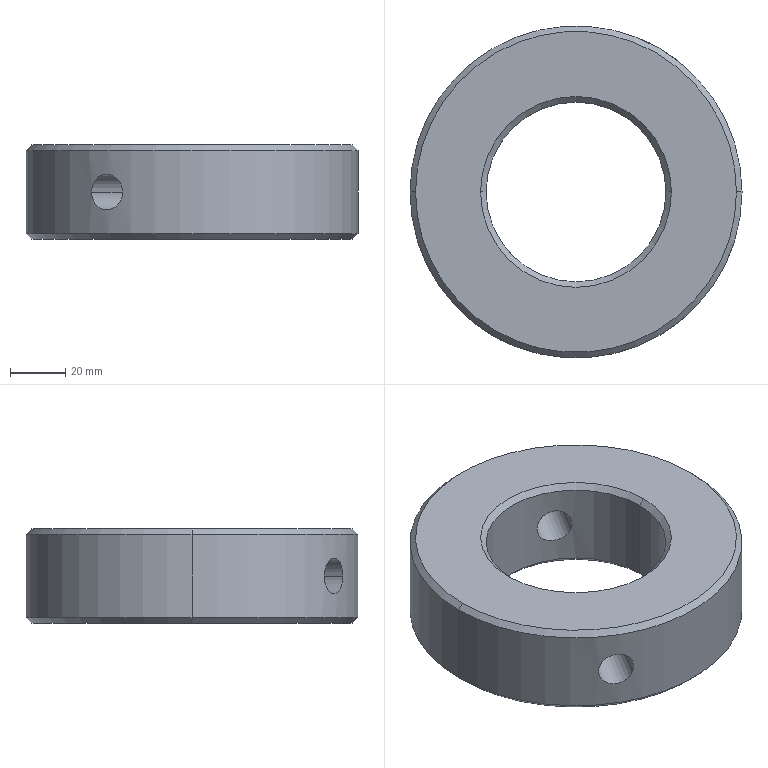Part | SolidWorks | features 3DProfileFeature 1, Chamfer 1, Extrusion 1, HoleWzd 1 | 1 solid | 18 faces | box 120 x 120 x 34 mm | volume 262064 mm3 | cone 8 | cylinder 8 | plane 2 | commonest cylinder face diameters 13 x4 65 x2 120 x2
STEP:
#1=CARTESIAN_POINT('',(-32.5,0.,32.));
#2=VERTEX_POINT('',#1);
#3=CARTESIAN_POINT('',(32.5,0.,32.));
#4=VERTEX_POINT('',#3);
#5=CARTESIAN_POINT('',(0.,0.,32.));
#6=DIRECTION('',(0.,0.,1.));
#7=DIRECTION('',(1.,0.,0.));
#8=AXIS2_PLACEMENT_3D('',#5,#6,#7);
#9=CIRCLE('',#8,32.5);
#10=EDGE_CURVE('',#2,#4,#9,.T.);
#11=ORIENTED_EDGE('',*,*,#10,.F.);
#12=CARTESIAN_POINT('',(-34.5,0.,34.));
#13=VERTEX_POINT('',#12);
#14=CARTESIAN_POINT('',(-32.5,0.,32.));
#15=DIRECTION('',(-0.7071,0.,0.7071));
#16=VECTOR('',#15,1000.);
#17=LINE('',#14,#16);
#18=EDGE_CURVE('',#2,#13,#17,.T.);
#19=ORIENTED_EDGE('',*,*,#18,.T.);
#20=CARTESIAN_POINT('',(34.5,0.,34.));
#21=VERTEX_POINT('',#20);
#22=CARTESIAN_POINT('',(0.,0.,34.));
#23=DIRECTION('',(0.,0.,-1.));
#24=DIRECTION('',(1.,0.,0.));
#25=AXIS2_PLACEMENT_3D('',#22,#23,#24);
#26=CIRCLE('',#25,34.5);
#27=EDGE_CURVE('',#21,#13,#26,.T.);
#28=ORIENTED_EDGE('',*,*,#27,.F.);
#29=CARTESIAN_POINT('',(32.5,0.,32.));
#30=DIRECTION('',(0.7071,0.,0.7071));
#31=VECTOR('',#30,1000.);
#32=LINE('',#29,#31);
#33=EDGE_CURVE('',#4,#21,#32,.T.);
#34=ORIENTED_EDGE('',*,*,#33,.F.);
#35=EDGE_LOOP('',(#11,#19,#28,#34));
#36=FACE_OUTER_BOUND('',#35,.T.);
#37=CARTESIAN_POINT('',(0.,0.,32.));
#38=DIRECTION('',(0.,0.,1.));
#39=DIRECTION('',(1.,0.,0.));
#40=AXIS2_PLACEMENT_3D('',#37,#38,#39);
#41=CONICAL_SURFACE('',#40,32.5,0.7854);
#42=ADVANCED_FACE('',(#36),#41,.F.);
#43=CARTESIAN_POINT('',(32.5,0.,2.));
#44=VERTEX_POINT('',#43);
#45=CARTESIAN_POINT('',(-32.5,0.,2.));
#46=VERTEX_POINT('',#45);
#47=CARTESIAN_POINT('',(0.,0.,2.));
#48=DIRECTION('',(0.,0.,-1.));
#49=DIRECTION('',(1.,0.,0.));
#50=AXIS2_PLACEMENT_3D('',#47,#48,#49);
#51=CIRCLE('',#50,32.5);
#52=EDGE_CURVE('',#44,#46,#51,.T.);
#53=ORIENTED_EDGE('',*,*,#52,.F.);
#54=CARTESIAN_POINT('',(34.5,0.,0.));
#55=VERTEX_POINT('',#54);
#56=CARTESIAN_POINT('',(34.5,0.,0.));
#57=DIRECTION('',(0.7071,0.,-0.7071));
#58=VECTOR('',#57,1000.);
#59=LINE('',#56,#58);
#60=EDGE_CURVE('',#44,#55,#59,.T.);
#61=ORIENTED_EDGE('',*,*,#60,.T.);
#62=CARTESIAN_POINT('',(-34.5,0.,0.));
#63=VERTEX_POINT('',#62);
#64=CARTESIAN_POINT('',(0.,0.,0.));
#65=DIRECTION('',(0.,0.,1.));
#66=DIRECTION('',(1.,0.,0.));
#67=AXIS2_PLACEMENT_3D('',#64,#65,#66);
#68=CIRCLE('',#67,34.5);
#69=EDGE_CURVE('',#63,#55,#68,.T.);
#70=ORIENTED_EDGE('',*,*,#69,.F.);
#71=CARTESIAN_POINT('',(-34.5,0.,0.));
#72=DIRECTION('',(-0.7071,0.,-0.7071));
#73=VECTOR('',#72,1000.);
#74=LINE('',#71,#73);
#75=EDGE_CURVE('',#46,#63,#74,.T.);
#76=ORIENTED_EDGE('',*,*,#75,.F.);
#77=EDGE_LOOP('',(#53,#61,#70,#76));
#78=FACE_OUTER_BOUND('',#77,.T.);
#79=CARTESIAN_POINT('',(0.,0.,0.));
#80=DIRECTION('',(0.,0.,-1.));
#81=DIRECTION('',(-1.,0.,0.));
#82=AXIS2_PLACEMENT_3D('',#79,#80,#81);
#83=CONICAL_SURFACE('',#82,34.5,0.7854);
#84=ADVANCED_FACE('',(#78),#83,.F.);
#85=CARTESIAN_POINT('',(58.,0.,34.));
#86=VERTEX_POINT('',#85);
#87=CARTESIAN_POINT('',(-58.,0.,34.));
#88=VERTEX_POINT('',#87);
#89=CARTESIAN_POINT('',(0.,0.,34.));
#90=DIRECTION('',(0.,0.,1.));
#91=DIRECTION('',(1.,0.,0.));
#92=AXIS2_PLACEMENT_3D('',#89,#90,#91);
#93=CIRCLE('',#92,58.);
#94=EDGE_CURVE('',#86,#88,#93,.T.);
#95=ORIENTED_EDGE('',*,*,#94,.F.);
#96=CARTESIAN_POINT('',(60.,0.,32.));
#97=VERTEX_POINT('',#96);
#98=CARTESIAN_POINT('',(58.,0.,34.));
#99=DIRECTION('',(0.7071,0.,-0.7071));
#100=VECTOR('',#99,1000.);
#101=LINE('',#98,#100);
#102=EDGE_CURVE('',#86,#97,#101,.T.);
#103=ORIENTED_EDGE('',*,*,#102,.T.);
#104=CARTESIAN_POINT('',(-60.,0.,32.));
#105=VERTEX_POINT('',#104);
#106=CARTESIAN_POINT('',(0.,0.,32.));
#107=DIRECTION('',(0.,0.,-1.));
#108=DIRECTION('',(1.,0.,0.));
#109=AXIS2_PLACEMENT_3D('',#106,#107,#108);
#110=CIRCLE('',#109,60.);
#111=EDGE_CURVE('',#105,#97,#110,.T.);
#112=ORIENTED_EDGE('',*,*,#111,.F.);
#113=CARTESIAN_POINT('',(-58.,0.,34.));
#114=DIRECTION('',(-0.7071,0.,-0.7071));
#115=VECTOR('',#114,1000.);
#116=LINE('',#113,#115);
#117=EDGE_CURVE('',#88,#105,#116,.T.);
#118=ORIENTED_EDGE('',*,*,#117,.F.);
#119=EDGE_LOOP('',(#95,#103,#112,#118));
#120=FACE_OUTER_BOUND('',#119,.T.);
#121=CARTESIAN_POINT('',(0.,0.,34.));
#122=DIRECTION('',(0.,0.,-1.));
#123=DIRECTION('',(-1.,0.,0.));
#124=AXIS2_PLACEMENT_3D('',#121,#122,#123);
#125=CONICAL_SURFACE('',#124,58.,0.7854);
#126=ADVANCED_FACE('',(#120),#125,.T.);
#127=CARTESIAN_POINT('',(-58.,0.,0.));
#128=VERTEX_POINT('',#127);
#129=CARTESIAN_POINT('',(58.,0.,0.));
#130=VERTEX_POINT('',#129);
#131=CARTESIAN_POINT('',(0.,0.,0.));
#132=DIRECTION('',(0.,0.,-1.));
#133=DIRECTION('',(1.,0.,0.));
#134=AXIS2_PLACEMENT_3D('',#131,#132,#133);
#135=CIRCLE('',#134,58.);
#136=EDGE_CURVE('',#128,#130,#135,.T.);
#137=ORIENTED_EDGE('',*,*,#136,.F.);
#138=CARTESIAN_POINT('',(-60.,0.,2.));
#139=VERTEX_POINT('',#138);
#140=CARTESIAN_POINT('',(-60.,0.,2.));
#141=DIRECTION('',(-0.7071,0.,0.7071));
#142=VECTOR('',#141,1000.);
#143=LINE('',#140,#142);
#144=EDGE_CURVE('',#128,#139,#143,.T.);
#145=ORIENTED_EDGE('',*,*,#144,.T.);
#146=CARTESIAN_POINT('',(60.,0.,2.));
#147=VERTEX_POINT('',#146);
#148=CARTESIAN_POINT('',(0.,0.,2.));
#149=DIRECTION('',(0.,0.,1.));
#150=DIRECTION('',(1.,0.,0.));
#151=AXIS2_PLACEMENT_3D('',#148,#149,#150);
#152=CIRCLE('',#151,60.);
#153=EDGE_CURVE('',#147,#139,#152,.T.);
#154=ORIENTED_EDGE('',*,*,#153,.F.);
#155=CARTESIAN_POINT('',(60.,0.,2.));
#156=DIRECTION('',(0.7071,0.,0.7071));
#157=VECTOR('',#156,1000.);
#158=LINE('',#155,#157);
#159=EDGE_CURVE('',#130,#147,#158,.T.);
#160=ORIENTED_EDGE('',*,*,#159,.F.);
#161=EDGE_LOOP('',(#137,#145,#154,#160));
#162=FACE_OUTER_BOUND('',#161,.T.);
#163=CARTESIAN_POINT('',(0.,0.,2.));
#164=DIRECTION('',(0.,0.,1.));
#165=DIRECTION('',(1.,0.,0.));
#166=AXIS2_PLACEMENT_3D('',#163,#164,#165);
#167=CONICAL_SURFACE('',#166,60.,0.7854);
#168=ADVANCED_FACE('',(#162),#167,.T.);
#169=CARTESIAN_POINT('',(-25.097,-54.499,17.));
#170=VERTEX_POINT('',#169);
#171=CARTESIAN_POINT('',(-36.247,-47.814,17.));
#172=VERTEX_POINT('',#171);
#173=CARTESIAN_POINT('',(-25.097,-54.499,17.));
#174=CARTESIAN_POINT('',(-25.097,-54.499,16.576));
#175=CARTESIAN_POINT('',(-25.135,-54.482,16.154));
#176=CARTESIAN_POINT('',(-25.249,-54.429,15.525));
#177=CARTESIAN_POINT('',(-25.297,-54.407,15.316));
#178=CARTESIAN_POINT('',(-25.409,-54.354,14.909));
#179=CARTESIAN_POINT('',(-25.54,-54.293,14.51));
#180=CARTESIAN_POINT('',(-25.704,-54.215,14.126));
#181=CARTESIAN_POINT('',(-25.886,-54.129,13.751));
#182=CARTESIAN_POINT('',(-25.986,-54.081,13.567));
#183=CARTESIAN_POINT('',(-26.308,-53.926,13.034));
#184=CARTESIAN_POINT('',(-26.55,-53.807,12.707));
#185=CARTESIAN_POINT('',(-27.087,-53.539,12.107));
#186=CARTESIAN_POINT('',(-27.385,-53.387,11.833));
#187=CARTESIAN_POINT('',(-28.013,-53.06,11.361));
#188=CARTESIAN_POINT('',(-28.343,-52.885,11.161));
#189=CARTESIAN_POINT('',(-28.861,-52.603,10.916));
#190=CARTESIAN_POINT('',(-29.039,-52.505,10.843));
#191=CARTESIAN_POINT('',(-29.396,-52.306,10.719));
#192=CARTESIAN_POINT('',(-29.575,-52.205,10.667));
#193=CARTESIAN_POINT('',(-30.117,-51.896,10.543));
#194=CARTESIAN_POINT('',(-30.481,-51.683,10.5));
#195=CARTESIAN_POINT('',(-31.218,-51.241,10.5));
#196=CARTESIAN_POINT('',(-31.578,-51.019,10.542));
#197=CARTESIAN_POINT('',(-32.106,-50.688,10.665));
#198=CARTESIAN_POINT('',(-32.28,-50.577,10.716));
#199=CARTESIAN_POINT('',(-32.624,-50.356,10.84));
#200=CARTESIAN_POINT('',(-32.794,-50.245,10.912));
#201=CARTESIAN_POINT('',(-33.288,-49.921,11.157));
#202=CARTESIAN_POINT('',(-33.598,-49.712,11.356));
#203=CARTESIAN_POINT('',(-34.182,-49.312,11.827));
#204=CARTESIAN_POINT('',(-34.457,-49.12,12.101));
#205=CARTESIAN_POINT('',(-34.948,-48.772,12.7));
#206=CARTESIAN_POINT('',(-35.167,-48.614,13.027));
#207=CARTESIAN_POINT('',(-35.456,-48.403,13.559));
#208=CARTESIAN_POINT('',(-35.546,-48.337,13.743));
#209=CARTESIAN_POINT('',(-35.708,-48.218,14.118));
#210=CARTESIAN_POINT('',(-35.781,-48.163,14.31));
#211=CARTESIAN_POINT('',(-35.978,-48.017,14.896));
#212=CARTESIAN_POINT('',(-36.078,-47.941,15.305));
#213=CARTESIAN_POINT('',(-36.213,-47.839,16.145));
#214=CARTESIAN_POINT('',(-36.247,-47.814,16.57));
#215=CARTESIAN_POINT('',(-36.247,-47.814,17.));
#216=B_SPLINE_CURVE_WITH_KNOTS('',3,(#173,#174,#175,#176,#177,#178,#179,#180,#181,#182,#183,#184,#185,#186,#187,#188,#189,#190,#191,#192,#193,#194,#195,#196,#197,#198,#199,#200,#201,#202,#203,#204,#205,#206,#207,#208,#209,#210,#211,#212,#213,#214,#215),.UNSPECIFIED.,.F.,.F.,(4,2,2,1,2,2,2,2,2,2,2,2,2,2,2,2,2,2,2,2,2,4),(0.02034,0.02161,0.02224,0.02288,0.02351,0.02415,0.02542,0.02669,0.02796,0.0286,0.02923,0.0305,0.03177,0.03241,0.03304,0.03432,0.03559,0.03686,0.03749,0.03813,0.0394,0.04067),.UNSPECIFIED.);
#217=EDGE_CURVE('',#170,#172,#216,.T.);
#218=ORIENTED_EDGE('',*,*,#217,.F.);
#219=CARTESIAN_POINT('',(-10.8,-30.653,17.));
#220=VERTEX_POINT('',#219);
#221=CARTESIAN_POINT('',(36.429,48.117,17.));
#222=DIRECTION('',(0.5142,0.8577,0.));
#223=VECTOR('',#222,1000.);
#224=LINE('',#221,#223);
#225=EDGE_CURVE('',#170,#220,#224,.T.);
#226=ORIENTED_EDGE('',*,*,#225,.T.);
#227=CARTESIAN_POINT('',(-21.95,-23.968,17.));
#228=VERTEX_POINT('',#227);
#229=CARTESIAN_POINT('',(-10.8,-30.653,17.));
#230=CARTESIAN_POINT('',(-10.8,-30.653,16.575));
#231=CARTESIAN_POINT('',(-10.84,-30.639,16.152));
#232=CARTESIAN_POINT('',(-11.001,-30.582,15.31));
#233=CARTESIAN_POINT('',(-11.12,-30.539,14.902));
#234=CARTESIAN_POINT('',(-11.352,-30.453,14.315));
#235=CARTESIAN_POINT('',(-11.439,-30.421,14.124));
#236=CARTESIAN_POINT('',(-11.629,-30.348,13.748));
#237=CARTESIAN_POINT('',(-11.734,-30.308,13.563));
#238=CARTESIAN_POINT('',(-12.069,-30.177,13.033));
#239=CARTESIAN_POINT('',(-12.321,-30.075,12.706));
#240=CARTESIAN_POINT('',(-12.879,-29.841,12.107));
#241=CARTESIAN_POINT('',(-13.187,-29.707,11.833));
#242=CARTESIAN_POINT('',(-13.831,-29.412,11.362));
#243=CARTESIAN_POINT('',(-14.169,-29.251,11.162));
#244=CARTESIAN_POINT('',(-14.7,-28.986,10.916));
#245=CARTESIAN_POINT('',(-14.881,-28.894,10.843));
#246=CARTESIAN_POINT('',(-15.243,-28.705,10.719));
#247=CARTESIAN_POINT('',(-15.424,-28.607,10.668));
#248=CARTESIAN_POINT('',(-15.972,-28.308,10.543));
#249=CARTESIAN_POINT('',(-16.342,-28.096,10.5));
#250=CARTESIAN_POINT('',(-17.078,-27.655,10.5));
#251=CARTESIAN_POINT('',(-17.436,-27.43,10.542));
#252=CARTESIAN_POINT('',(-18.134,-26.974,10.707));
#253=CARTESIAN_POINT('',(-18.477,-26.74,10.833));
#254=CARTESIAN_POINT('',(-19.119,-26.284,11.158));
#255=CARTESIAN_POINT('',(-19.421,-26.062,11.357));
#256=CARTESIAN_POINT('',(-19.845,-25.738,11.712));
#257=CARTESIAN_POINT('',(-19.983,-25.631,11.84));
#258=CARTESIAN_POINT('',(-20.243,-25.426,12.11));
#259=CARTESIAN_POINT('',(-20.367,-25.327,12.252));
#260=CARTESIAN_POINT('',(-20.719,-25.042,12.7));
#261=CARTESIAN_POINT('',(-20.928,-24.866,13.026));
#262=CARTESIAN_POINT('',(-21.295,-24.552,13.738));
#263=CARTESIAN_POINT('',(-21.448,-24.418,14.112));
#264=CARTESIAN_POINT('',(-21.634,-24.254,14.698));
#265=CARTESIAN_POINT('',(-21.688,-24.205,14.898));
#266=CARTESIAN_POINT('',(-21.783,-24.12,15.306));
#267=CARTESIAN_POINT('',(-21.823,-24.084,15.515));
#268=CARTESIAN_POINT('',(-21.918,-23.997,16.145));
#269=CARTESIAN_POINT('',(-21.95,-23.968,16.569));
#270=CARTESIAN_POINT('',(-21.95,-23.968,17.));
#271=B_SPLINE_CURVE_WITH_KNOTS('',3,(#229,#230,#231,#232,#233,#234,#235,#236,#237,#238,#239,#240,#241,#242,#243,#244,#245,#246,#247,#248,#249,#250,#251,#252,#253,#254,#255,#256,#257,#258,#259,#260,#261,#262,#263,#264,#265,#266,#267,#268,#269,#270),.UNSPECIFIED.,.F.,.F.,(4,2,2,2,2,2,2,2,2,2,2,2,2,2,2,2,2,2,2,2,4),(0.02037,0.02165,0.02292,0.02356,0.02419,0.02547,0.02674,0.02801,0.02865,0.02928,0.03056,0.03183,0.0331,0.03438,0.03501,0.03565,0.03692,0.0382,0.03883,0.03947,0.04074),.UNSPECIFIED.);
#272=EDGE_CURVE('',#220,#228,#271,.T.);
#273=ORIENTED_EDGE('',*,*,#272,.T.);
#274=CARTESIAN_POINT('',(25.279,54.802,17.));
#275=DIRECTION('',(0.5142,0.8577,0.));
#276=VECTOR('',#275,1000.);
#277=LINE('',#274,#276);
#278=EDGE_CURVE('',#172,#228,#277,.T.);
#279=ORIENTED_EDGE('',*,*,#278,.F.);
#280=EDGE_LOOP('',(#218,#226,#273,#279));
#281=FACE_OUTER_BOUND('',#280,.T.);
#282=CARTESIAN_POINT('',(30.854,51.459,17.));
#283=DIRECTION('',(0.5142,0.8577,0.));
#284=DIRECTION('',(-0.8577,0.5142,0.));
#285=AXIS2_PLACEMENT_3D('',#282,#283,#284);
#286=CYLINDRICAL_SURFACE('',#285,6.5);
#287=ADVANCED_FACE('',(#281),#286,.F.);
#288=CARTESIAN_POINT('',(10.8,30.653,17.));
#289=VERTEX_POINT('',#288);
#290=CARTESIAN_POINT('',(21.95,23.968,17.));
#291=VERTEX_POINT('',#290);
#292=CARTESIAN_POINT('',(10.8,30.653,17.));
#293=CARTESIAN_POINT('',(10.8,30.653,16.569));
#294=CARTESIAN_POINT('',(10.841,30.639,16.146));
#295=CARTESIAN_POINT('',(10.96,30.596,15.522));
#296=CARTESIAN_POINT('',(11.01,30.578,15.316));
#297=CARTESIAN_POINT('',(11.129,30.535,14.907));
#298=CARTESIAN_POINT('',(11.199,30.51,14.704));
#299=CARTESIAN_POINT('',(11.432,30.423,14.114));
#300=CARTESIAN_POINT('',(11.622,30.352,13.741));
#301=CARTESIAN_POINT('',(12.068,30.177,13.035));
#302=CARTESIAN_POINT('',(12.325,30.074,12.702));
#303=CARTESIAN_POINT('',(12.882,29.84,12.104));
#304=CARTESIAN_POINT('',(13.184,29.708,11.835));
#305=CARTESIAN_POINT('',(13.834,29.411,11.36));
#306=CARTESIAN_POINT('',(14.176,29.248,11.159));
#307=CARTESIAN_POINT('',(14.702,28.985,10.915));
#308=CARTESIAN_POINT('',(14.88,28.894,10.844));
#309=CARTESIAN_POINT('',(15.242,28.705,10.72));
#310=CARTESIAN_POINT('',(15.426,28.606,10.667));
#311=CARTESIAN_POINT('',(15.979,28.304,10.542));
#312=CARTESIAN_POINT('',(16.346,28.094,10.5));
#313=CARTESIAN_POINT('',(17.075,27.656,10.5));
#314=CARTESIAN_POINT('',(17.441,27.427,10.542));
#315=CARTESIAN_POINT('',(18.14,26.97,10.709));
#316=CARTESIAN_POINT('',(18.476,26.741,10.832));
#317=CARTESIAN_POINT('',(18.959,26.398,11.077));
#318=CARTESIAN_POINT('',(19.118,26.283,11.169));
#319=CARTESIAN_POINT('',(19.421,26.059,11.37));
#320=CARTESIAN_POINT('',(19.567,25.95,11.48));
#321=CARTESIAN_POINT('',(19.989,25.628,11.832));
#322=CARTESIAN_POINT('',(20.25,25.422,12.102));
#323=CARTESIAN_POINT('',(20.724,25.037,12.706));
#324=CARTESIAN_POINT('',(20.932,24.863,13.034));
#325=CARTESIAN_POINT('',(21.204,24.631,13.561));
#326=CARTESIAN_POINT('',(21.288,24.558,13.743));
#327=CARTESIAN_POINT('',(21.442,24.423,14.119));
#328=CARTESIAN_POINT('',(21.512,24.361,14.314));
#329=CARTESIAN_POINT('',(21.698,24.196,14.903));
#330=CARTESIAN_POINT('',(21.791,24.112,15.308));
#331=CARTESIAN_POINT('',(21.886,24.026,15.935));
#332=CARTESIAN_POINT('',(21.91,24.004,16.148));
#333=CARTESIAN_POINT('',(21.942,23.975,16.575));
#334=CARTESIAN_POINT('',(21.95,23.968,16.788));
#335=CARTESIAN_POINT('',(21.95,23.968,17.));
#336=B_SPLINE_CURVE_WITH_KNOTS('',3,(#292,#293,#294,#295,#296,#297,#298,#299,#300,#301,#302,#303,#304,#305,#306,#307,#308,#309,#310,#311,#312,#313,#314,#315,#316,#317,#318,#319,#320,#321,#322,#323,#324,#325,#326,#327,#328,#329,#330,#331,#332,#333,#334,#335),.UNSPECIFIED.,.F.,.F.,(4,2,2,2,2,2,2,2,2,2,2,2,2,2,2,2,2,2,2,2,2,4),(0.,0.001273,0.00191,0.002547,0.00382,0.005093,0.006367,0.00764,0.008277,0.008913,0.01019,0.01146,0.01273,0.01337,0.01401,0.01528,0.01655,0.01719,0.01783,0.0191,0.01974,0.02037),.UNSPECIFIED.);
#337=EDGE_CURVE('',#289,#291,#336,.T.);
#338=ORIENTED_EDGE('',*,*,#337,.T.);
#339=CARTESIAN_POINT('',(36.247,47.814,17.));
#340=VERTEX_POINT('',#339);
#341=CARTESIAN_POINT('',(36.429,48.117,17.));
#342=DIRECTION('',(0.5142,0.8577,0.));
#343=VECTOR('',#342,1000.);
#344=LINE('',#341,#343);
#345=EDGE_CURVE('',#291,#340,#344,.T.);
#346=ORIENTED_EDGE('',*,*,#345,.T.);
#347=CARTESIAN_POINT('',(25.097,54.499,17.));
#348=VERTEX_POINT('',#347);
#349=CARTESIAN_POINT('',(25.097,54.499,17.));
#350=CARTESIAN_POINT('',(25.097,54.499,16.57));
#351=CARTESIAN_POINT('',(25.136,54.481,16.148));
#352=CARTESIAN_POINT('',(25.249,54.429,15.524));
#353=CARTESIAN_POINT('',(25.296,54.407,15.318));
#354=CARTESIAN_POINT('',(25.409,54.354,14.91));
#355=CARTESIAN_POINT('',(25.475,54.323,14.707));
#356=CARTESIAN_POINT('',(25.698,54.218,14.116));
#357=CARTESIAN_POINT('',(25.879,54.132,13.743));
#358=CARTESIAN_POINT('',(26.306,53.926,13.037));
#359=CARTESIAN_POINT('',(26.553,53.805,12.702));
#360=CARTESIAN_POINT('',(27.091,53.537,12.103));
#361=CARTESIAN_POINT('',(27.383,53.388,11.834));
#362=CARTESIAN_POINT('',(27.857,53.142,11.478));
#363=CARTESIAN_POINT('',(28.02,53.056,11.367));
#364=CARTESIAN_POINT('',(28.352,52.879,11.167));
#365=CARTESIAN_POINT('',(28.69,52.698,10.986));
#366=CARTESIAN_POINT('',(29.039,52.505,10.843));
#367=CARTESIAN_POINT('',(29.395,52.307,10.719));
#368=CARTESIAN_POINT('',(29.577,52.204,10.667));
#369=CARTESIAN_POINT('',(30.124,51.892,10.541));
#370=CARTESIAN_POINT('',(30.488,51.679,10.5));
#371=CARTESIAN_POINT('',(31.216,51.242,10.5));
#372=CARTESIAN_POINT('',(31.583,51.017,10.542));
#373=CARTESIAN_POINT('',(32.289,50.573,10.708));
#374=CARTESIAN_POINT('',(32.63,50.353,10.831));
#375=CARTESIAN_POINT('',(33.124,50.028,11.076));
#376=CARTESIAN_POINT('',(33.286,49.92,11.168));
#377=CARTESIAN_POINT('',(33.599,49.71,11.369));
#378=CARTESIAN_POINT('',(33.75,49.608,11.478));
#379=CARTESIAN_POINT('',(34.186,49.309,11.831));
#380=CARTESIAN_POINT('',(34.456,49.121,12.1));
#381=CARTESIAN_POINT('',(34.953,48.769,12.707));
#382=CARTESIAN_POINT('',(35.171,48.611,13.035));
#383=CARTESIAN_POINT('',(35.458,48.402,13.562));
#384=CARTESIAN_POINT('',(35.546,48.337,13.744));
#385=CARTESIAN_POINT('',(35.709,48.217,14.12));
#386=CARTESIAN_POINT('',(35.783,48.162,14.315));
#387=CARTESIAN_POINT('',(35.981,48.015,14.906));
#388=CARTESIAN_POINT('',(36.079,47.94,15.311));
#389=CARTESIAN_POINT('',(36.213,47.84,16.145));
#390=CARTESIAN_POINT('',(36.247,47.814,16.576));
#391=CARTESIAN_POINT('',(36.247,47.814,17.));
#392=B_SPLINE_CURVE_WITH_KNOTS('',3,(#349,#350,#351,#352,#353,#354,#355,#356,#357,#358,#359,#360,#361,#362,#363,#364,#365,#366,#367,#368,#369,#370,#371,#372,#373,#374,#375,#376,#377,#378,#379,#380,#381,#382,#383,#384,#385,#386,#387,#388,#389,#390,#391),.UNSPECIFIED.,.F.,.F.,(4,2,2,2,2,2,2,2,1,2,2,2,2,2,2,2,2,2,2,2,2,4),(0.,0.001271,0.001907,0.002542,0.003813,0.005084,0.006355,0.006991,0.007626,0.008262,0.008897,0.01017,0.01144,0.01271,0.01335,0.01398,0.01525,0.01652,0.01716,0.01779,0.01907,0.02034),.UNSPECIFIED.);
#393=EDGE_CURVE('',#348,#340,#392,.T.);
#394=ORIENTED_EDGE('',*,*,#393,.F.);
#395=CARTESIAN_POINT('',(25.279,54.802,17.));
#396=DIRECTION('',(0.5142,0.8577,0.));
#397=VECTOR('',#396,1000.);
#398=LINE('',#395,#397);
#399=EDGE_CURVE('',#289,#348,#398,.T.);
#400=ORIENTED_EDGE('',*,*,#399,.F.);
#401=EDGE_LOOP('',(#338,#346,#394,#400));
#402=FACE_OUTER_BOUND('',#401,.T.);
#403=CARTESIAN_POINT('',(30.854,51.459,17.));
#404=DIRECTION('',(0.5142,0.8577,0.));
#405=DIRECTION('',(-0.8577,0.5142,0.));
#406=AXIS2_PLACEMENT_3D('',#403,#404,#405);
#407=CYLINDRICAL_SURFACE('',#406,6.5);
#408=ADVANCED_FACE('',(#402),#407,.F.);
#409=CARTESIAN_POINT('',(-21.95,-23.968,17.));
#410=CARTESIAN_POINT('',(-21.95,-23.968,17.431));
#411=CARTESIAN_POINT('',(-21.918,-23.997,17.854));
#412=CARTESIAN_POINT('',(-21.824,-24.083,18.478));
#413=CARTESIAN_POINT('',(-21.785,-24.118,18.684));
#414=CARTESIAN_POINT('',(-21.691,-24.203,19.093));
#415=CARTESIAN_POINT('',(-21.635,-24.252,19.296));
#416=CARTESIAN_POINT('',(-21.449,-24.418,19.886));
#417=CARTESIAN_POINT('',(-21.296,-24.551,20.259));
#418=CARTESIAN_POINT('',(-20.933,-24.862,20.965));
#419=CARTESIAN_POINT('',(-20.72,-25.04,21.298));
#420=CARTESIAN_POINT('',(-20.251,-25.421,21.896));
#421=CARTESIAN_POINT('',(-19.993,-25.625,22.165));
#422=CARTESIAN_POINT('',(-19.425,-26.059,22.64));
#423=CARTESIAN_POINT('',(-19.12,-26.284,22.841));
#424=CARTESIAN_POINT('',(-18.64,-26.624,23.085));
#425=CARTESIAN_POINT('',(-18.476,-26.738,23.156));
#426=CARTESIAN_POINT('',(-18.139,-26.968,23.28));
#427=CARTESIAN_POINT('',(-17.965,-27.084,23.333));
#428=CARTESIAN_POINT('',(-17.437,-27.429,23.458));
#429=CARTESIAN_POINT('',(-17.079,-27.654,23.5));
#430=CARTESIAN_POINT('',(-16.35,-28.091,23.5));
#431=CARTESIAN_POINT('',(-15.975,-28.306,23.458));
#432=CARTESIAN_POINT('',(-15.243,-28.707,23.291));
#433=CARTESIAN_POINT('',(-14.882,-28.895,23.168));
#434=CARTESIAN_POINT('',(-14.352,-29.16,22.923));
#435=CARTESIAN_POINT('',(-14.176,-29.246,22.831));
#436=CARTESIAN_POINT('',(-13.836,-29.408,22.63));
#437=CARTESIAN_POINT('',(-13.67,-29.486,22.52));
#438=CARTESIAN_POINT('',(-13.188,-29.706,22.168));
#439=CARTESIAN_POINT('',(-12.883,-29.839,21.898));
#440=CARTESIAN_POINT('',(-12.321,-30.076,21.294));
#441=CARTESIAN_POINT('',(-12.069,-30.177,20.966));
#442=CARTESIAN_POINT('',(-11.736,-30.307,20.439));
#443=CARTESIAN_POINT('',(-11.632,-30.347,20.257));
#444=CARTESIAN_POINT('',(-11.441,-30.42,19.881));
#445=CARTESIAN_POINT('',(-11.353,-30.453,19.686));
#446=CARTESIAN_POINT('',(-11.12,-30.539,19.097));
#447=CARTESIAN_POINT('',(-11.001,-30.581,18.692));
#448=CARTESIAN_POINT('',(-10.881,-30.624,18.065));
#449=CARTESIAN_POINT('',(-10.851,-30.635,17.852));
#450=CARTESIAN_POINT('',(-10.81,-30.65,17.425));
#451=CARTESIAN_POINT('',(-10.8,-30.653,17.212));
#452=CARTESIAN_POINT('',(-10.8,-30.653,17.));
#453=B_SPLINE_CURVE_WITH_KNOTS('',3,(#409,#410,#411,#412,#413,#414,#415,#416,#417,#418,#419,#420,#421,#422,#423,#424,#425,#426,#427,#428,#429,#430,#431,#432,#433,#434,#435,#436,#437,#438,#439,#440,#441,#442,#443,#444,#445,#446,#447,#448,#449,#450,#451,#452),.UNSPECIFIED.,.F.,.F.,(4,2,2,2,2,2,2,2,2,2,2,2,2,2,2,2,2,2,2,2,2,4),(0.,0.001273,0.00191,0.002547,0.00382,0.005093,0.006367,0.00764,0.008277,0.008913,0.01019,0.01146,0.01273,0.01337,0.01401,0.01528,0.01655,0.01719,0.01783,0.0191,0.01974,0.02037),.UNSPECIFIED.);
#454=EDGE_CURVE('',#228,#220,#453,.T.);
#455=ORIENTED_EDGE('',*,*,#454,.F.);
#456=ORIENTED_EDGE('',*,*,#272,.F.);
#457=EDGE_LOOP('',(#455,#456));
#458=FACE_BOUND('',#457,.T.);
#459=ORIENTED_EDGE('',*,*,#10,.T.);
#460=CARTESIAN_POINT('',(32.5,0.,34.));
#461=DIRECTION('',(0.,0.,-1.));
#462=VECTOR('',#461,1000.);
#463=LINE('',#460,#462);
#464=EDGE_CURVE('',#4,#44,#463,.T.);
#465=ORIENTED_EDGE('',*,*,#464,.T.);
#466=ORIENTED_EDGE('',*,*,#52,.T.);
#467=CARTESIAN_POINT('',(-32.5,0.,34.));
#468=DIRECTION('',(0.,0.,-1.));
#469=VECTOR('',#468,1000.);
#470=LINE('',#467,#469);
#471=EDGE_CURVE('',#2,#46,#470,.T.);
#472=ORIENTED_EDGE('',*,*,#471,.F.);
#473=EDGE_LOOP('',(#459,#465,#466,#472));
#474=FACE_OUTER_BOUND('',#473,.T.);
#475=CARTESIAN_POINT('',(0.,0.,34.));
#476=DIRECTION('',(0.,0.,-1.));
#477=DIRECTION('',(-1.,0.,0.));
#478=AXIS2_PLACEMENT_3D('',#475,#476,#477);
#479=CYLINDRICAL_SURFACE('',#478,32.5);
#480=ADVANCED_FACE('',(#458,#474),#479,.F.);
#481=ORIENTED_EDGE('',*,*,#393,.T.);
#482=CARTESIAN_POINT('',(36.247,47.814,17.));
#483=CARTESIAN_POINT('',(36.247,47.814,17.424));
#484=CARTESIAN_POINT('',(36.214,47.839,17.846));
#485=CARTESIAN_POINT('',(36.114,47.915,18.475));
#486=CARTESIAN_POINT('',(36.072,47.946,18.684));
#487=CARTESIAN_POINT('',(35.972,48.021,19.091));
#488=CARTESIAN_POINT('',(35.857,48.107,19.49));
#489=CARTESIAN_POINT('',(35.711,48.215,19.874));
#490=CARTESIAN_POINT('',(35.549,48.335,20.249));
#491=CARTESIAN_POINT('',(35.46,48.4,20.433));
#492=CARTESIAN_POINT('',(35.171,48.611,20.966));
#493=CARTESIAN_POINT('',(34.953,48.769,21.293));
#494=CARTESIAN_POINT('',(34.463,49.116,21.893));
#495=CARTESIAN_POINT('',(34.188,49.308,22.167));
#496=CARTESIAN_POINT('',(33.605,49.708,22.639));
#497=CARTESIAN_POINT('',(33.295,49.916,22.839));
#498=CARTESIAN_POINT('',(32.802,50.24,23.084));
#499=CARTESIAN_POINT('',(32.631,50.351,23.157));
#500=CARTESIAN_POINT('',(32.288,50.572,23.281));
#501=CARTESIAN_POINT('',(32.114,50.683,23.333));
#502=CARTESIAN_POINT('',(31.586,51.015,23.457));
#503=CARTESIAN_POINT('',(31.226,51.236,23.5));
#504=CARTESIAN_POINT('',(30.49,51.678,23.5));
#505=CARTESIAN_POINT('',(30.125,51.891,23.458));
#506=CARTESIAN_POINT('',(29.583,52.2,23.335));
#507=CARTESIAN_POINT('',(29.404,52.302,23.284));
#508=CARTESIAN_POINT('',(29.047,52.501,23.16));
#509=CARTESIAN_POINT('',(28.869,52.599,23.088));
#510=CARTESIAN_POINT('',(28.35,52.881,22.843));
#511=CARTESIAN_POINT('',(28.02,53.057,22.644));
#512=CARTESIAN_POINT('',(27.392,53.384,22.173));
#513=CARTESIAN_POINT('',(27.093,53.536,21.899));
#514=CARTESIAN_POINT('',(26.555,53.804,21.3));
#515=CARTESIAN_POINT('',(26.312,53.923,20.973));
#516=CARTESIAN_POINT('',(25.99,54.079,20.441));
#517=CARTESIAN_POINT('',(25.89,54.127,20.257));
#518=CARTESIAN_POINT('',(25.708,54.214,19.882));
#519=CARTESIAN_POINT('',(25.625,54.253,19.69));
#520=CARTESIAN_POINT('',(25.404,54.357,19.104));
#521=CARTESIAN_POINT('',(25.289,54.41,18.695));
#522=CARTESIAN_POINT('',(25.136,54.481,17.855));
#523=CARTESIAN_POINT('',(25.097,54.499,17.43));
#524=CARTESIAN_POINT('',(25.097,54.499,17.));
#525=B_SPLINE_CURVE_WITH_KNOTS('',3,(#482,#483,#484,#485,#486,#487,#488,#489,#490,#491,#492,#493,#494,#495,#496,#497,#498,#499,#500,#501,#502,#503,#504,#505,#506,#507,#508,#509,#510,#511,#512,#513,#514,#515,#516,#517,#518,#519,#520,#521,#522,#523,#524),.UNSPECIFIED.,.F.,.F.,(4,2,2,1,2,2,2,2,2,2,2,2,2,2,2,2,2,2,2,2,2,4),(0.02034,0.02161,0.02224,0.02288,0.02351,0.02415,0.02542,0.02669,0.02796,0.0286,0.02923,0.0305,0.03177,0.03241,0.03304,0.03432,0.03559,0.03686,0.03749,0.03813,0.0394,0.04067),.UNSPECIFIED.);
#526=EDGE_CURVE('',#340,#348,#525,.T.);
#527=ORIENTED_EDGE('',*,*,#526,.T.);
#528=EDGE_LOOP('',(#481,#527));
#529=FACE_BOUND('',#528,.T.);
#530=ORIENTED_EDGE('',*,*,#111,.T.);
#531=CARTESIAN_POINT('',(60.,0.,34.));
#532=DIRECTION('',(0.,0.,-1.));
#533=VECTOR('',#532,1000.);
#534=LINE('',#531,#533);
#535=EDGE_CURVE('',#97,#147,#534,.T.);
#536=ORIENTED_EDGE('',*,*,#535,.T.);
#537=ORIENTED_EDGE('',*,*,#153,.T.);
#538=CARTESIAN_POINT('',(-60.,0.,34.));
#539=DIRECTION('',(0.,0.,-1.));
#540=VECTOR('',#539,1000.);
#541=LINE('',#538,#540);
#542=EDGE_CURVE('',#105,#139,#541,.T.);
#543=ORIENTED_EDGE('',*,*,#542,.F.);
#544=EDGE_LOOP('',(#530,#536,#537,#543));
#545=FACE_OUTER_BOUND('',#544,.T.);
#546=CARTESIAN_POINT('',(0.,0.,34.));
#547=DIRECTION('',(0.,0.,-1.));
#548=DIRECTION('',(-1.,0.,0.));
#549=AXIS2_PLACEMENT_3D('',#546,#547,#548);
#550=CYLINDRICAL_SURFACE('',#549,60.);
#551=ADVANCED_FACE('',(#529,#545),#550,.T.);
#552=CARTESIAN_POINT('',(0.,0.,34.));
#553=DIRECTION('',(0.,0.,1.));
#554=DIRECTION('',(1.,0.,0.));
#555=AXIS2_PLACEMENT_3D('',#552,#553,#554);
#556=CIRCLE('',#555,58.);
#557=EDGE_CURVE('',#88,#86,#556,.T.);
#558=ORIENTED_EDGE('',*,*,#557,.T.);
#559=ORIENTED_EDGE('',*,*,#94,.T.);
#560=EDGE_LOOP('',(#558,#559));
#561=FACE_OUTER_BOUND('',#560,.T.);
#562=ORIENTED_EDGE('',*,*,#27,.T.);
#563=CARTESIAN_POINT('',(0.,0.,34.));
#564=DIRECTION('',(0.,0.,-1.));
#565=DIRECTION('',(1.,0.,0.));
#566=AXIS2_PLACEMENT_3D('',#563,#564,#565);
#567=CIRCLE('',#566,34.5);
#568=EDGE_CURVE('',#13,#21,#567,.T.);
#569=ORIENTED_EDGE('',*,*,#568,.T.);
#570=EDGE_LOOP('',(#562,#569));
#571=FACE_BOUND('',#570,.T.);
#572=CARTESIAN_POINT('',(0.,0.,34.));
#573=DIRECTION('',(0.,0.,1.));
#574=DIRECTION('',(1.,0.,0.));
#575=AXIS2_PLACEMENT_3D('',#572,#573,#574);
#576=PLANE('',#575);
#577=ADVANCED_FACE('',(#561,#571),#576,.T.);
#578=CARTESIAN_POINT('',(0.,0.,0.));
#579=DIRECTION('',(0.,0.,-1.));
#580=DIRECTION('',(1.,0.,0.));
#581=AXIS2_PLACEMENT_3D('',#578,#579,#580);
#582=CIRCLE('',#581,58.);
#583=EDGE_CURVE('',#130,#128,#582,.T.);
#584=ORIENTED_EDGE('',*,*,#583,.T.);
#585=ORIENTED_EDGE('',*,*,#136,.T.);
#586=EDGE_LOOP('',(#584,#585));
#587=FACE_OUTER_BOUND('',#586,.T.);
#588=ORIENTED_EDGE('',*,*,#69,.T.);
#589=CARTESIAN_POINT('',(0.,0.,0.));
#590=DIRECTION('',(0.,0.,1.));
#591=DIRECTION('',(1.,0.,0.));
#592=AXIS2_PLACEMENT_3D('',#589,#590,#591);
#593=CIRCLE('',#592,34.5);
#594=EDGE_CURVE('',#55,#63,#593,.T.);
#595=ORIENTED_EDGE('',*,*,#594,.T.);
#596=EDGE_LOOP('',(#588,#595));
#597=FACE_BOUND('',#596,.T.);
#598=CARTESIAN_POINT('',(0.,0.,0.));
#599=DIRECTION('',(0.,0.,1.));
#600=DIRECTION('',(1.,0.,0.));
#601=AXIS2_PLACEMENT_3D('',#598,#599,#600);
#602=PLANE('',#601);
#603=ADVANCED_FACE('',(#587,#597),#602,.F.);
#604=ORIENTED_EDGE('',*,*,#535,.F.);
#605=CARTESIAN_POINT('',(0.,0.,32.));
#606=DIRECTION('',(0.,0.,-1.));
#607=DIRECTION('',(1.,0.,0.));
#608=AXIS2_PLACEMENT_3D('',#605,#606,#607);
#609=CIRCLE('',#608,60.);
#610=EDGE_CURVE('',#97,#105,#609,.T.);
#611=ORIENTED_EDGE('',*,*,#610,.T.);
#612=ORIENTED_EDGE('',*,*,#542,.T.);
#613=CARTESIAN_POINT('',(0.,0.,2.));
#614=DIRECTION('',(0.,0.,1.));
#615=DIRECTION('',(1.,0.,0.));
#616=AXIS2_PLACEMENT_3D('',#613,#614,#615);
#617=CIRCLE('',#616,60.);
#618=EDGE_CURVE('',#139,#147,#617,.T.);
#619=ORIENTED_EDGE('',*,*,#618,.T.);
#620=EDGE_LOOP('',(#604,#611,#612,#619));
#621=FACE_OUTER_BOUND('',#620,.T.);
#622=CARTESIAN_POINT('',(-36.247,-47.814,17.));
#623=CARTESIAN_POINT('',(-36.247,-47.814,17.43));
#624=CARTESIAN_POINT('',(-36.213,-47.839,17.852));
#625=CARTESIAN_POINT('',(-36.114,-47.915,18.476));
#626=CARTESIAN_POINT('',(-36.072,-47.946,18.682));
#627=CARTESIAN_POINT('',(-35.973,-48.021,19.09));
#628=CARTESIAN_POINT('',(-35.914,-48.064,19.293));
#629=CARTESIAN_POINT('',(-35.717,-48.211,19.884));
#630=CARTESIAN_POINT('',(-35.556,-48.331,20.257));
#631=CARTESIAN_POINT('',(-35.173,-48.61,20.963));
#632=CARTESIAN_POINT('',(-34.95,-48.771,21.298));
#633=CARTESIAN_POINT('',(-34.459,-49.119,21.897));
#634=CARTESIAN_POINT('',(-34.19,-49.307,22.166));
#635=CARTESIAN_POINT('',(-33.75,-49.608,22.522));
#636=CARTESIAN_POINT('',(-33.597,-49.712,22.633));
#637=CARTESIAN_POINT('',(-33.285,-49.921,22.833));
#638=CARTESIAN_POINT('',(-32.966,-50.134,23.014));
#639=CARTESIAN_POINT('',(-32.631,-50.351,23.157));
#640=CARTESIAN_POINT('',(-32.289,-50.572,23.281));
#641=CARTESIAN_POINT('',(-32.112,-50.684,23.333));
#642=CARTESIAN_POINT('',(-31.579,-51.019,23.459));
#643=CARTESIAN_POINT('',(-31.22,-51.24,23.5));
#644=CARTESIAN_POINT('',(-30.492,-51.676,23.5));
#645=CARTESIAN_POINT('',(-30.12,-51.894,23.458));
#646=CARTESIAN_POINT('',(-29.396,-52.307,23.292));
#647=CARTESIAN_POINT('',(-29.041,-52.505,23.169));
#648=CARTESIAN_POINT('',(-28.522,-52.788,22.924));
#649=CARTESIAN_POINT('',(-28.35,-52.88,22.832));
#650=CARTESIAN_POINT('',(-28.018,-53.057,22.631));
#651=CARTESIAN_POINT('',(-27.857,-53.142,22.522));
#652=CARTESIAN_POINT('',(-27.387,-53.386,22.169));
#653=CARTESIAN_POINT('',(-27.094,-53.535,21.9));
#654=CARTESIAN_POINT('',(-26.55,-53.807,21.293));
#655=CARTESIAN_POINT('',(-26.307,-53.926,20.965));
#656=CARTESIAN_POINT('',(-25.988,-54.08,20.438));
#657=CARTESIAN_POINT('',(-25.889,-54.127,20.256));
#658=CARTESIAN_POINT('',(-25.707,-54.214,19.88));
#659=CARTESIAN_POINT('',(-25.623,-54.254,19.685));
#660=CARTESIAN_POINT('',(-25.4,-54.359,19.094));
#661=CARTESIAN_POINT('',(-25.288,-54.411,18.689));
#662=CARTESIAN_POINT('',(-25.136,-54.481,17.855));
#663=CARTESIAN_POINT('',(-25.097,-54.499,17.424));
#664=CARTESIAN_POINT('',(-25.097,-54.499,17.));
#665=B_SPLINE_CURVE_WITH_KNOTS('',3,(#622,#623,#624,#625,#626,#627,#628,#629,#630,#631,#632,#633,#634,#635,#636,#637,#638,#639,#640,#641,#642,#643,#644,#645,#646,#647,#648,#649,#650,#651,#652,#653,#654,#655,#656,#657,#658,#659,#660,#661,#662,#663,#664),.UNSPECIFIED.,.F.,.F.,(4,2,2,2,2,2,2,2,1,2,2,2,2,2,2,2,2,2,2,2,2,4),(0.,0.001271,0.001907,0.002542,0.003813,0.005084,0.006355,0.006991,0.007626,0.008262,0.008897,0.01017,0.01144,0.01271,0.01335,0.01398,0.01525,0.01652,0.01716,0.01779,0.01907,0.02034),.UNSPECIFIED.);
#666=EDGE_CURVE('',#172,#170,#665,.T.);
#667=ORIENTED_EDGE('',*,*,#666,.T.);
#668=ORIENTED_EDGE('',*,*,#217,.T.);
#669=EDGE_LOOP('',(#667,#668));
#670=FACE_BOUND('',#669,.T.);
#671=CARTESIAN_POINT('',(0.,0.,34.));
#672=DIRECTION('',(0.,0.,-1.));
#673=DIRECTION('',(-1.,0.,0.));
#674=AXIS2_PLACEMENT_3D('',#671,#672,#673);
#675=CYLINDRICAL_SURFACE('',#674,60.);
#676=ADVANCED_FACE('',(#621,#670),#675,.T.);
#677=ORIENTED_EDGE('',*,*,#464,.F.);
#678=CARTESIAN_POINT('',(0.,0.,32.));
#679=DIRECTION('',(0.,0.,1.));
#680=DIRECTION('',(1.,0.,0.));
#681=AXIS2_PLACEMENT_3D('',#678,#679,#680);
#682=CIRCLE('',#681,32.5);
#683=EDGE_CURVE('',#4,#2,#682,.T.);
#684=ORIENTED_EDGE('',*,*,#683,.T.);
#685=ORIENTED_EDGE('',*,*,#471,.T.);
#686=CARTESIAN_POINT('',(0.,0.,2.));
#687=DIRECTION('',(0.,0.,-1.));
#688=DIRECTION('',(1.,0.,0.));
#689=AXIS2_PLACEMENT_3D('',#686,#687,#688);
#690=CIRCLE('',#689,32.5);
#691=EDGE_CURVE('',#46,#44,#690,.T.);
#692=ORIENTED_EDGE('',*,*,#691,.T.);
#693=EDGE_LOOP('',(#677,#684,#685,#692));
#694=FACE_OUTER_BOUND('',#693,.T.);
#695=ORIENTED_EDGE('',*,*,#337,.F.);
#696=CARTESIAN_POINT('',(21.95,23.968,17.));
#697=CARTESIAN_POINT('',(21.95,23.968,17.425));
#698=CARTESIAN_POINT('',(21.919,23.997,17.848));
#699=CARTESIAN_POINT('',(21.792,24.111,18.69));
#700=CARTESIAN_POINT('',(21.698,24.197,19.098));
#701=CARTESIAN_POINT('',(21.513,24.361,19.685));
#702=CARTESIAN_POINT('',(21.444,24.422,19.876));
#703=CARTESIAN_POINT('',(21.29,24.556,20.252));
#704=CARTESIAN_POINT('',(21.205,24.63,20.437));
#705=CARTESIAN_POINT('',(20.931,24.863,20.967));
#706=CARTESIAN_POINT('',(20.723,25.038,21.294));
#707=CARTESIAN_POINT('',(20.254,25.419,21.893));
#708=CARTESIAN_POINT('',(19.99,25.628,22.167));
#709=CARTESIAN_POINT('',(19.427,26.057,22.638));
#710=CARTESIAN_POINT('',(19.126,26.279,22.838));
#711=CARTESIAN_POINT('',(18.642,26.623,23.084));
#712=CARTESIAN_POINT('',(18.475,26.739,23.157));
#713=CARTESIAN_POINT('',(18.138,26.969,23.281));
#714=CARTESIAN_POINT('',(17.967,27.083,23.332));
#715=CARTESIAN_POINT('',(17.444,27.425,23.457));
#716=CARTESIAN_POINT('',(17.083,27.651,23.5));
#717=CARTESIAN_POINT('',(16.347,28.093,23.5));
#718=CARTESIAN_POINT('',(15.98,28.303,23.458));
#719=CARTESIAN_POINT('',(15.249,28.703,23.293));
#720=CARTESIAN_POINT('',(14.881,28.896,23.167));
#721=CARTESIAN_POINT('',(14.177,29.248,22.842));
#722=CARTESIAN_POINT('',(13.838,29.409,22.643));
#723=CARTESIAN_POINT('',(13.353,29.631,22.288));
#724=CARTESIAN_POINT('',(13.194,29.702,22.16));
#725=CARTESIAN_POINT('',(12.89,29.835,21.89));
#726=CARTESIAN_POINT('',(12.744,29.897,21.748));
#727=CARTESIAN_POINT('',(12.327,30.073,21.3));
#728=CARTESIAN_POINT('',(12.074,30.175,20.974));
#729=CARTESIAN_POINT('',(11.623,30.351,20.262));
#730=CARTESIAN_POINT('',(11.433,30.423,19.888));
#731=CARTESIAN_POINT('',(11.201,30.509,19.302));
#732=CARTESIAN_POINT('',(11.132,30.534,19.102));
#733=CARTESIAN_POINT('',(11.012,30.577,18.694));
#734=CARTESIAN_POINT('',(10.962,30.596,18.485));
#735=CARTESIAN_POINT('',(10.841,30.639,17.855));
#736=CARTESIAN_POINT('',(10.8,30.653,17.431));
#737=CARTESIAN_POINT('',(10.8,30.653,17.));
#738=B_SPLINE_CURVE_WITH_KNOTS('',3,(#696,#697,#698,#699,#700,#701,#702,#703,#704,#705,#706,#707,#708,#709,#710,#711,#712,#713,#714,#715,#716,#717,#718,#719,#720,#721,#722,#723,#724,#725,#726,#727,#728,#729,#730,#731,#732,#733,#734,#735,#736,#737),.UNSPECIFIED.,.F.,.F.,(4,2,2,2,2,2,2,2,2,2,2,2,2,2,2,2,2,2,2,2,4),(0.02037,0.02165,0.02292,0.02356,0.02419,0.02547,0.02674,0.02801,0.02865,0.02928,0.03056,0.03183,0.0331,0.03438,0.03501,0.03565,0.03692,0.0382,0.03883,0.03947,0.04074),.UNSPECIFIED.);
#739=EDGE_CURVE('',#291,#289,#738,.T.);
#740=ORIENTED_EDGE('',*,*,#739,.F.);
#741=EDGE_LOOP('',(#695,#740));
#742=FACE_BOUND('',#741,.T.);
#743=CARTESIAN_POINT('',(0.,0.,34.));
#744=DIRECTION('',(0.,0.,-1.));
#745=DIRECTION('',(-1.,0.,0.));
#746=AXIS2_PLACEMENT_3D('',#743,#744,#745);
#747=CYLINDRICAL_SURFACE('',#746,32.5);
#748=ADVANCED_FACE('',(#694,#742),#747,.F.);
#749=ORIENTED_EDGE('',*,*,#345,.F.);
#750=ORIENTED_EDGE('',*,*,#739,.T.);
#751=ORIENTED_EDGE('',*,*,#399,.T.);
#752=ORIENTED_EDGE('',*,*,#526,.F.);
#753=EDGE_LOOP('',(#749,#750,#751,#752));
#754=FACE_OUTER_BOUND('',#753,.T.);
#755=CARTESIAN_POINT('',(30.854,51.459,17.));
#756=DIRECTION('',(0.5142,0.8577,0.));
#757=DIRECTION('',(-0.8577,0.5142,0.));
#758=AXIS2_PLACEMENT_3D('',#755,#756,#757);
#759=CYLINDRICAL_SURFACE('',#758,6.5);
#760=ADVANCED_FACE('',(#754),#759,.F.);
#761=ORIENTED_EDGE('',*,*,#225,.F.);
#762=ORIENTED_EDGE('',*,*,#666,.F.);
#763=ORIENTED_EDGE('',*,*,#278,.T.);
#764=ORIENTED_EDGE('',*,*,#454,.T.);
#765=EDGE_LOOP('',(#761,#762,#763,#764));
#766=FACE_OUTER_BOUND('',#765,.T.);
#767=CARTESIAN_POINT('',(30.854,51.459,17.));
#768=DIRECTION('',(0.5142,0.8577,0.));
#769=DIRECTION('',(-0.8577,0.5142,0.));
#770=AXIS2_PLACEMENT_3D('',#767,#768,#769);
#771=CYLINDRICAL_SURFACE('',#770,6.5);
#772=ADVANCED_FACE('',(#766),#771,.F.);
#773=ORIENTED_EDGE('',*,*,#144,.F.);
#774=ORIENTED_EDGE('',*,*,#583,.F.);
#775=ORIENTED_EDGE('',*,*,#159,.T.);
#776=ORIENTED_EDGE('',*,*,#618,.F.);
#777=EDGE_LOOP('',(#773,#774,#775,#776));
#778=FACE_OUTER_BOUND('',#777,.T.);
#779=CARTESIAN_POINT('',(0.,0.,2.));
#780=DIRECTION('',(0.,0.,1.));
#781=DIRECTION('',(1.,0.,0.));
#782=AXIS2_PLACEMENT_3D('',#779,#780,#781);
#783=CONICAL_SURFACE('',#782,60.,0.7854);
#784=ADVANCED_FACE('',(#778),#783,.T.);
#785=ORIENTED_EDGE('',*,*,#102,.F.);
#786=ORIENTED_EDGE('',*,*,#557,.F.);
#787=ORIENTED_EDGE('',*,*,#117,.T.);
#788=ORIENTED_EDGE('',*,*,#610,.F.);
#789=EDGE_LOOP('',(#785,#786,#787,#788));
#790=FACE_OUTER_BOUND('',#789,.T.);
#791=CARTESIAN_POINT('',(0.,0.,34.));
#792=DIRECTION('',(0.,0.,-1.));
#793=DIRECTION('',(-1.,0.,0.));
#794=AXIS2_PLACEMENT_3D('',#791,#792,#793);
#795=CONICAL_SURFACE('',#794,58.,0.7854);
#796=ADVANCED_FACE('',(#790),#795,.T.);
#797=ORIENTED_EDGE('',*,*,#60,.F.);
#798=ORIENTED_EDGE('',*,*,#691,.F.);
#799=ORIENTED_EDGE('',*,*,#75,.T.);
#800=ORIENTED_EDGE('',*,*,#594,.F.);
#801=EDGE_LOOP('',(#797,#798,#799,#800));
#802=FACE_OUTER_BOUND('',#801,.T.);
#803=CARTESIAN_POINT('',(0.,0.,0.));
#804=DIRECTION('',(0.,0.,-1.));
#805=DIRECTION('',(-1.,0.,0.));
#806=AXIS2_PLACEMENT_3D('',#803,#804,#805);
#807=CONICAL_SURFACE('',#806,34.5,0.7854);
#808=ADVANCED_FACE('',(#802),#807,.F.);
#809=ORIENTED_EDGE('',*,*,#18,.F.);
#810=ORIENTED_EDGE('',*,*,#683,.F.);
#811=ORIENTED_EDGE('',*,*,#33,.T.);
#812=ORIENTED_EDGE('',*,*,#568,.F.);
#813=EDGE_LOOP('',(#809,#810,#811,#812));
#814=FACE_OUTER_BOUND('',#813,.T.);
#815=CARTESIAN_POINT('',(0.,0.,32.));
#816=DIRECTION('',(0.,0.,1.));
#817=DIRECTION('',(1.,0.,0.));
#818=AXIS2_PLACEMENT_3D('',#815,#816,#817);
#819=CONICAL_SURFACE('',#818,32.5,0.7854);
#820=ADVANCED_FACE('',(#814),#819,.F.);
#821=CLOSED_SHELL('',(#42,#84,#126,#168,#287,#408,#480,#551,#577,#603,#676,#748,#760,#772,#784,#796,#808,#820));
#822=MANIFOLD_SOLID_BREP('',#821);
#823=CARTESIAN_POINT('',(0.,0.,0.));
#824=DIRECTION('',(0.,0.,1.));
#825=DIRECTION('',(1.,0.,0.));
#826=AXIS2_PLACEMENT_3D('',#823,#824,#825);
#827=(LENGTH_UNIT()NAMED_UNIT(*)SI_UNIT(.MILLI.,.METRE.));
#828=UNCERTAINTY_MEASURE_WITH_UNIT(LENGTH_MEASURE(0.00001),#827,'','');
#829=(NAMED_UNIT(*)PLANE_ANGLE_UNIT()SI_UNIT($,.RADIAN.));
#830=(NAMED_UNIT(*)SI_UNIT($,.STERADIAN.)SOLID_ANGLE_UNIT());
#831=(GEOMETRIC_REPRESENTATION_CONTEXT(3)GLOBAL_UNCERTAINTY_ASSIGNED_CONTEXT((#828))GLOBAL_UNIT_ASSIGNED_CONTEXT((#827,#829,#830))REPRESENTATION_CONTEXT('',''));
#832=ADVANCED_BREP_SHAPE_REPRESENTATION('',(#822,#826),#831);